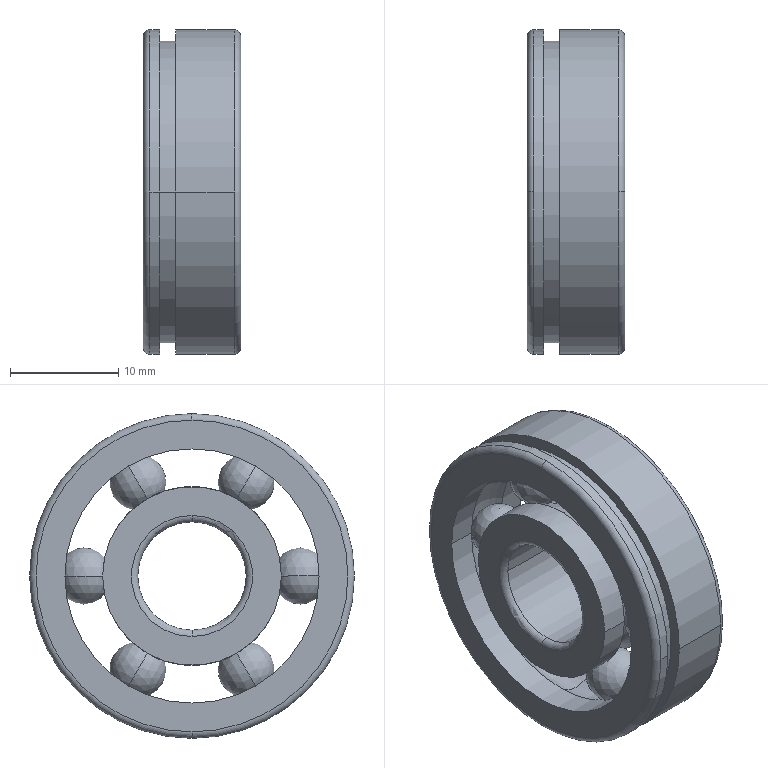Part | SolidWorks | features BaseBody 8 | 8 solids | 48 faces | box 9 x 30 x 30 mm | volume 3673 mm3 | cylinder 16 | torus 14 | sphere 12 | plane 6 | commonest cylinder face diameters 16.52 x4 23.48 x4 30 x4 10 x2 27.84 x2
STEP:
#1=CARTESIAN_POINT('',(4.5,7.4,0.));
#2=VERTEX_POINT('',#1);
#3=CARTESIAN_POINT('',(4.5,12.6,0.));
#4=VERTEX_POINT('',#3);
#5=CARTESIAN_POINT('',(4.5,10.,0.));
#6=DIRECTION('',(0.,0.,1.));
#7=DIRECTION('',(1.,0.,0.));
#8=AXIS2_PLACEMENT_3D('',#5,#6,#7);
#9=CIRCLE('',#8,2.6);
#10=EDGE_CURVE('',#2,#4,#9,.T.);
#11=ORIENTED_EDGE('',*,*,#10,.F.);
#12=CARTESIAN_POINT('',(4.5,10.,0.));
#13=DIRECTION('',(0.,0.,-1.));
#14=DIRECTION('',(-1.,0.,0.));
#15=AXIS2_PLACEMENT_3D('',#12,#13,#14);
#16=CIRCLE('',#15,2.6);
#17=EDGE_CURVE('',#2,#4,#16,.T.);
#18=ORIENTED_EDGE('',*,*,#17,.T.);
#19=EDGE_LOOP('',(#11,#18));
#20=FACE_OUTER_BOUND('',#19,.T.);
#21=CARTESIAN_POINT('',(4.5,10.,0.));
#22=DIRECTION('',(0.,0.,-1.));
#23=DIRECTION('',(1.,0.,0.));
#24=AXIS2_PLACEMENT_3D('',#21,#22,#23);
#25=SPHERICAL_SURFACE('',#24,2.6);
#26=ADVANCED_FACE('',(#20),#25,.T.);
#27=ORIENTED_EDGE('',*,*,#17,.F.);
#28=ORIENTED_EDGE('',*,*,#10,.T.);
#29=EDGE_LOOP('',(#27,#28));
#30=FACE_OUTER_BOUND('',#29,.T.);
#31=CARTESIAN_POINT('',(4.5,10.,0.));
#32=DIRECTION('',(0.,0.,-1.));
#33=DIRECTION('',(1.,0.,0.));
#34=AXIS2_PLACEMENT_3D('',#31,#32,#33);
#35=SPHERICAL_SURFACE('',#34,2.6);
#36=ADVANCED_FACE('',(#30),#35,.T.);
#37=CLOSED_SHELL('',(#26,#36));
#38=MANIFOLD_SOLID_BREP('',#37);
#39=CARTESIAN_POINT('',(3.,-13.92,0.));
#40=VERTEX_POINT('',#39);
#41=CARTESIAN_POINT('',(3.,13.92,0.));
#42=VERTEX_POINT('',#41);
#43=CARTESIAN_POINT('',(3.,0.,0.));
#44=DIRECTION('',(1.,0.,0.));
#45=DIRECTION('',(0.,1.,0.));
#46=AXIS2_PLACEMENT_3D('',#43,#44,#45);
#47=CIRCLE('',#46,13.92);
#48=EDGE_CURVE('',#40,#42,#47,.T.);
#49=ORIENTED_EDGE('',*,*,#48,.F.);
#50=CARTESIAN_POINT('',(1.5,-13.92,0.));
#51=VERTEX_POINT('',#50);
#52=CARTESIAN_POINT('',(2.25,-13.92,0.));
#53=DIRECTION('',(-1.,0.,0.));
#54=VECTOR('',#53,1000.);
#55=LINE('',#52,#54);
#56=EDGE_CURVE('',#40,#51,#55,.T.);
#57=ORIENTED_EDGE('',*,*,#56,.T.);
#58=CARTESIAN_POINT('',(1.5,13.92,0.));
#59=VERTEX_POINT('',#58);
#60=CARTESIAN_POINT('',(1.5,0.,0.));
#61=DIRECTION('',(1.,0.,0.));
#62=DIRECTION('',(0.,1.,0.));
#63=AXIS2_PLACEMENT_3D('',#60,#61,#62);
#64=CIRCLE('',#63,13.92);
#65=EDGE_CURVE('',#51,#59,#64,.T.);
#66=ORIENTED_EDGE('',*,*,#65,.T.);
#67=CARTESIAN_POINT('',(2.25,13.92,0.));
#68=DIRECTION('',(-1.,0.,0.));
#69=VECTOR('',#68,1000.);
#70=LINE('',#67,#69);
#71=EDGE_CURVE('',#42,#59,#70,.T.);
#72=ORIENTED_EDGE('',*,*,#71,.F.);
#73=EDGE_LOOP('',(#49,#57,#66,#72));
#74=FACE_OUTER_BOUND('',#73,.T.);
#75=CARTESIAN_POINT('',(2.25,0.,0.));
#76=DIRECTION('',(-1.,0.,0.));
#77=DIRECTION('',(0.,1.,0.));
#78=AXIS2_PLACEMENT_3D('',#75,#76,#77);
#79=CYLINDRICAL_SURFACE('',#78,13.92);
#80=ADVANCED_FACE('',(#74),#79,.T.);
#81=CARTESIAN_POINT('',(8.4,-15.,0.));
#82=VERTEX_POINT('',#81);
#83=CARTESIAN_POINT('',(8.4,0.,-15.));
#84=VERTEX_POINT('',#83);
#85=CARTESIAN_POINT('',(8.4,0.,0.));
#86=DIRECTION('',(1.,0.,0.));
#87=DIRECTION('',(0.,-1.,0.));
#88=AXIS2_PLACEMENT_3D('',#85,#86,#87);
#89=CIRCLE('',#88,15.);
#90=EDGE_CURVE('',#82,#84,#89,.T.);
#91=ORIENTED_EDGE('',*,*,#90,.F.);
#92=CARTESIAN_POINT('',(3.,-15.,0.));
#93=VERTEX_POINT('',#92);
#94=CARTESIAN_POINT('',(6.,-15.,0.));
#95=DIRECTION('',(-1.,0.,0.));
#96=VECTOR('',#95,1000.);
#97=LINE('',#94,#96);
#98=EDGE_CURVE('',#82,#93,#97,.T.);
#99=ORIENTED_EDGE('',*,*,#98,.T.);
#100=CARTESIAN_POINT('',(3.,15.,0.));
#101=VERTEX_POINT('',#100);
#102=CARTESIAN_POINT('',(3.,0.,0.));
#103=DIRECTION('',(1.,0.,0.));
#104=DIRECTION('',(0.,1.,0.));
#105=AXIS2_PLACEMENT_3D('',#102,#103,#104);
#106=CIRCLE('',#105,15.);
#107=EDGE_CURVE('',#93,#101,#106,.T.);
#108=ORIENTED_EDGE('',*,*,#107,.T.);
#109=CARTESIAN_POINT('',(8.4,15.,0.));
#110=VERTEX_POINT('',#109);
#111=CARTESIAN_POINT('',(6.,15.,0.));
#112=DIRECTION('',(-1.,0.,0.));
#113=VECTOR('',#112,1000.);
#114=LINE('',#111,#113);
#115=EDGE_CURVE('',#110,#101,#114,.T.);
#116=ORIENTED_EDGE('',*,*,#115,.F.);
#117=CARTESIAN_POINT('',(8.4,0.,0.));
#118=DIRECTION('',(1.,0.,0.));
#119=DIRECTION('',(0.,-1.,0.));
#120=AXIS2_PLACEMENT_3D('',#117,#118,#119);
#121=CIRCLE('',#120,15.);
#122=EDGE_CURVE('',#84,#110,#121,.T.);
#123=ORIENTED_EDGE('',*,*,#122,.F.);
#124=EDGE_LOOP('',(#91,#99,#108,#116,#123));
#125=FACE_OUTER_BOUND('',#124,.T.);
#126=CARTESIAN_POINT('',(6.,0.,0.));
#127=DIRECTION('',(-1.,0.,0.));
#128=DIRECTION('',(0.,1.,0.));
#129=AXIS2_PLACEMENT_3D('',#126,#127,#128);
#130=CYLINDRICAL_SURFACE('',#129,15.);
#131=ADVANCED_FACE('',(#125),#130,.T.);
#132=CARTESIAN_POINT('',(1.5,-15.,0.));
#133=VERTEX_POINT('',#132);
#134=CARTESIAN_POINT('',(1.5,15.,0.));
#135=VERTEX_POINT('',#134);
#136=CARTESIAN_POINT('',(1.5,0.,0.));
#137=DIRECTION('',(1.,0.,0.));
#138=DIRECTION('',(0.,1.,0.));
#139=AXIS2_PLACEMENT_3D('',#136,#137,#138);
#140=CIRCLE('',#139,15.);
#141=EDGE_CURVE('',#133,#135,#140,.T.);
#142=ORIENTED_EDGE('',*,*,#141,.F.);
#143=CARTESIAN_POINT('',(0.6,-15.,0.));
#144=VERTEX_POINT('',#143);
#145=CARTESIAN_POINT('',(0.75,-15.,0.));
#146=DIRECTION('',(-1.,0.,0.));
#147=VECTOR('',#146,1000.);
#148=LINE('',#145,#147);
#149=EDGE_CURVE('',#133,#144,#148,.T.);
#150=ORIENTED_EDGE('',*,*,#149,.T.);
#151=CARTESIAN_POINT('',(0.6,0.,-15.));
#152=VERTEX_POINT('',#151);
#153=CARTESIAN_POINT('',(0.6,0.,0.));
#154=DIRECTION('',(-1.,0.,0.));
#155=DIRECTION('',(0.,-1.,0.));
#156=AXIS2_PLACEMENT_3D('',#153,#154,#155);
#157=CIRCLE('',#156,15.);
#158=EDGE_CURVE('',#152,#144,#157,.T.);
#159=ORIENTED_EDGE('',*,*,#158,.F.);
#160=CARTESIAN_POINT('',(0.6,15.,0.));
#161=VERTEX_POINT('',#160);
#162=CARTESIAN_POINT('',(0.6,0.,0.));
#163=DIRECTION('',(-1.,0.,0.));
#164=DIRECTION('',(0.,-1.,0.));
#165=AXIS2_PLACEMENT_3D('',#162,#163,#164);
#166=CIRCLE('',#165,15.);
#167=EDGE_CURVE('',#161,#152,#166,.T.);
#168=ORIENTED_EDGE('',*,*,#167,.F.);
#169=CARTESIAN_POINT('',(0.75,15.,0.));
#170=DIRECTION('',(-1.,0.,0.));
#171=VECTOR('',#170,1000.);
#172=LINE('',#169,#171);
#173=EDGE_CURVE('',#135,#161,#172,.T.);
#174=ORIENTED_EDGE('',*,*,#173,.F.);
#175=EDGE_LOOP('',(#142,#150,#159,#168,#174));
#176=FACE_OUTER_BOUND('',#175,.T.);
#177=CARTESIAN_POINT('',(0.75,0.,0.));
#178=DIRECTION('',(-1.,0.,0.));
#179=DIRECTION('',(0.,1.,0.));
#180=AXIS2_PLACEMENT_3D('',#177,#178,#179);
#181=CYLINDRICAL_SURFACE('',#180,15.);
#182=ADVANCED_FACE('',(#176),#181,.T.);
#183=ORIENTED_EDGE('',*,*,#122,.T.);
#184=CARTESIAN_POINT('',(8.4,0.,15.));
#185=VERTEX_POINT('',#184);
#186=CARTESIAN_POINT('',(8.4,0.,0.));
#187=DIRECTION('',(1.,0.,0.));
#188=DIRECTION('',(0.,-1.,0.));
#189=AXIS2_PLACEMENT_3D('',#186,#187,#188);
#190=CIRCLE('',#189,15.);
#191=EDGE_CURVE('',#110,#185,#190,.T.);
#192=ORIENTED_EDGE('',*,*,#191,.T.);
#193=CARTESIAN_POINT('',(9.,0.,14.4));
#194=VERTEX_POINT('',#193);
#195=CARTESIAN_POINT('',(8.4,0.,14.4));
#196=DIRECTION('',(0.,1.,0.));
#197=DIRECTION('',(0.,0.,1.));
#198=AXIS2_PLACEMENT_3D('',#195,#196,#197);
#199=CIRCLE('',#198,0.6);
#200=EDGE_CURVE('',#185,#194,#199,.T.);
#201=ORIENTED_EDGE('',*,*,#200,.T.);
#202=CARTESIAN_POINT('',(9.,0.,-14.4));
#203=VERTEX_POINT('',#202);
#204=CARTESIAN_POINT('',(9.,0.,0.));
#205=DIRECTION('',(-1.,0.,0.));
#206=DIRECTION('',(0.,-1.,0.));
#207=AXIS2_PLACEMENT_3D('',#204,#205,#206);
#208=CIRCLE('',#207,14.4);
#209=EDGE_CURVE('',#194,#203,#208,.T.);
#210=ORIENTED_EDGE('',*,*,#209,.T.);
#211=CARTESIAN_POINT('',(8.4,0.,-14.4));
#212=DIRECTION('',(0.,-1.,0.));
#213=DIRECTION('',(0.,0.,-1.));
#214=AXIS2_PLACEMENT_3D('',#211,#212,#213);
#215=CIRCLE('',#214,0.6);
#216=EDGE_CURVE('',#84,#203,#215,.T.);
#217=ORIENTED_EDGE('',*,*,#216,.F.);
#218=EDGE_LOOP('',(#183,#192,#201,#210,#217));
#219=FACE_OUTER_BOUND('',#218,.T.);
#220=CARTESIAN_POINT('',(8.4,0.,0.));
#221=DIRECTION('',(1.,0.,0.));
#222=DIRECTION('',(0.,0.,-1.));
#223=AXIS2_PLACEMENT_3D('',#220,#221,#222);
#224=TOROIDAL_SURFACE('',#223,14.4,0.6);
#225=ADVANCED_FACE('',(#219),#224,.T.);
#226=CARTESIAN_POINT('',(0.,0.,-14.4));
#227=VERTEX_POINT('',#226);
#228=CARTESIAN_POINT('',(0.,0.,14.4));
#229=VERTEX_POINT('',#228);
#230=CARTESIAN_POINT('',(0.,0.,0.));
#231=DIRECTION('',(1.,0.,0.));
#232=DIRECTION('',(0.,-1.,0.));
#233=AXIS2_PLACEMENT_3D('',#230,#231,#232);
#234=CIRCLE('',#233,14.4);
#235=EDGE_CURVE('',#227,#229,#234,.T.);
#236=ORIENTED_EDGE('',*,*,#235,.T.);
#237=CARTESIAN_POINT('',(0.6,0.,15.));
#238=VERTEX_POINT('',#237);
#239=CARTESIAN_POINT('',(0.6,0.,14.4));
#240=DIRECTION('',(0.,1.,0.));
#241=DIRECTION('',(0.,0.,1.));
#242=AXIS2_PLACEMENT_3D('',#239,#240,#241);
#243=CIRCLE('',#242,0.6);
#244=EDGE_CURVE('',#229,#238,#243,.T.);
#245=ORIENTED_EDGE('',*,*,#244,.T.);
#246=CARTESIAN_POINT('',(0.6,0.,0.));
#247=DIRECTION('',(-1.,0.,0.));
#248=DIRECTION('',(0.,-1.,0.));
#249=AXIS2_PLACEMENT_3D('',#246,#247,#248);
#250=CIRCLE('',#249,15.);
#251=EDGE_CURVE('',#238,#161,#250,.T.);
#252=ORIENTED_EDGE('',*,*,#251,.T.);
#253=ORIENTED_EDGE('',*,*,#167,.T.);
#254=CARTESIAN_POINT('',(0.6,0.,-14.4));
#255=DIRECTION('',(0.,-1.,0.));
#256=DIRECTION('',(0.,0.,-1.));
#257=AXIS2_PLACEMENT_3D('',#254,#255,#256);
#258=CIRCLE('',#257,0.6);
#259=EDGE_CURVE('',#227,#152,#258,.T.);
#260=ORIENTED_EDGE('',*,*,#259,.F.);
#261=EDGE_LOOP('',(#236,#245,#252,#253,#260));
#262=FACE_OUTER_BOUND('',#261,.T.);
#263=CARTESIAN_POINT('',(0.6,0.,0.));
#264=DIRECTION('',(1.,0.,0.));
#265=DIRECTION('',(0.,0.,-1.));
#266=AXIS2_PLACEMENT_3D('',#263,#264,#265);
#267=TOROIDAL_SURFACE('',#266,14.4,0.6);
#268=ADVANCED_FACE('',(#262),#267,.T.);
#269=CARTESIAN_POINT('',(2.568,0.,11.74));
#270=VERTEX_POINT('',#269);
#271=CARTESIAN_POINT('',(2.568,-11.74,0.));
#272=VERTEX_POINT('',#271);
#273=CARTESIAN_POINT('',(2.568,0.,0.));
#274=DIRECTION('',(1.,0.,0.));
#275=DIRECTION('',(0.,1.,0.));
#276=AXIS2_PLACEMENT_3D('',#273,#274,#275);
#277=CIRCLE('',#276,11.74);
#278=EDGE_CURVE('',#270,#272,#277,.T.);
#279=ORIENTED_EDGE('',*,*,#278,.F.);
#280=CARTESIAN_POINT('',(6.432,0.,11.74));
#281=VERTEX_POINT('',#280);
#282=CARTESIAN_POINT('',(4.5,0.,10.));
#283=DIRECTION('',(0.,1.,0.));
#284=DIRECTION('',(0.,0.,1.));
#285=AXIS2_PLACEMENT_3D('',#282,#283,#284);
#286=CIRCLE('',#285,2.6);
#287=EDGE_CURVE('',#270,#281,#286,.T.);
#288=ORIENTED_EDGE('',*,*,#287,.T.);
#289=CARTESIAN_POINT('',(6.432,-11.74,0.));
#290=VERTEX_POINT('',#289);
#291=CARTESIAN_POINT('',(6.432,0.,0.));
#292=DIRECTION('',(1.,0.,0.));
#293=DIRECTION('',(0.,1.,0.));
#294=AXIS2_PLACEMENT_3D('',#291,#292,#293);
#295=CIRCLE('',#294,11.74);
#296=EDGE_CURVE('',#281,#290,#295,.T.);
#297=ORIENTED_EDGE('',*,*,#296,.T.);
#298=CARTESIAN_POINT('',(6.432,0.,-11.74));
#299=VERTEX_POINT('',#298);
#300=CARTESIAN_POINT('',(6.432,0.,0.));
#301=DIRECTION('',(1.,0.,0.));
#302=DIRECTION('',(0.,1.,0.));
#303=AXIS2_PLACEMENT_3D('',#300,#301,#302);
#304=CIRCLE('',#303,11.74);
#305=EDGE_CURVE('',#290,#299,#304,.T.);
#306=ORIENTED_EDGE('',*,*,#305,.T.);
#307=CARTESIAN_POINT('',(2.568,0.,-11.74));
#308=VERTEX_POINT('',#307);
#309=CARTESIAN_POINT('',(4.5,0.,-10.));
#310=DIRECTION('',(0.,-1.,0.));
#311=DIRECTION('',(0.,0.,-1.));
#312=AXIS2_PLACEMENT_3D('',#309,#310,#311);
#313=CIRCLE('',#312,2.6);
#314=EDGE_CURVE('',#308,#299,#313,.T.);
#315=ORIENTED_EDGE('',*,*,#314,.F.);
#316=CARTESIAN_POINT('',(2.568,0.,0.));
#317=DIRECTION('',(1.,0.,0.));
#318=DIRECTION('',(0.,1.,0.));
#319=AXIS2_PLACEMENT_3D('',#316,#317,#318);
#320=CIRCLE('',#319,11.74);
#321=EDGE_CURVE('',#272,#308,#320,.T.);
#322=ORIENTED_EDGE('',*,*,#321,.F.);
#323=EDGE_LOOP('',(#279,#288,#297,#306,#315,#322));
#324=FACE_OUTER_BOUND('',#323,.T.);
#325=CARTESIAN_POINT('',(4.5,0.,0.));
#326=DIRECTION('',(1.,0.,0.));
#327=DIRECTION('',(0.,0.,-1.));
#328=AXIS2_PLACEMENT_3D('',#325,#326,#327);
#329=TOROIDAL_SURFACE('',#328,10.,2.6);
#330=ADVANCED_FACE('',(#324),#329,.F.);
#331=CARTESIAN_POINT('',(9.,11.74,0.));
#332=VERTEX_POINT('',#331);
#333=CARTESIAN_POINT('',(9.,-11.74,0.));
#334=VERTEX_POINT('',#333);
#335=CARTESIAN_POINT('',(9.,0.,0.));
#336=DIRECTION('',(1.,0.,0.));
#337=DIRECTION('',(0.,1.,0.));
#338=AXIS2_PLACEMENT_3D('',#335,#336,#337);
#339=CIRCLE('',#338,11.74);
#340=EDGE_CURVE('',#332,#334,#339,.T.);
#341=ORIENTED_EDGE('',*,*,#340,.T.);
#342=CARTESIAN_POINT('',(7.716,-11.74,0.));
#343=DIRECTION('',(-1.,0.,0.));
#344=VECTOR('',#343,1000.);
#345=LINE('',#342,#344);
#346=EDGE_CURVE('',#334,#290,#345,.T.);
#347=ORIENTED_EDGE('',*,*,#346,.T.);
#348=ORIENTED_EDGE('',*,*,#296,.F.);
#349=CARTESIAN_POINT('',(6.432,11.74,0.));
#350=VERTEX_POINT('',#349);
#351=CARTESIAN_POINT('',(6.432,0.,0.));
#352=DIRECTION('',(1.,0.,0.));
#353=DIRECTION('',(0.,1.,0.));
#354=AXIS2_PLACEMENT_3D('',#351,#352,#353);
#355=CIRCLE('',#354,11.74);
#356=EDGE_CURVE('',#350,#281,#355,.T.);
#357=ORIENTED_EDGE('',*,*,#356,.F.);
#358=CARTESIAN_POINT('',(7.716,11.74,0.));
#359=DIRECTION('',(-1.,0.,0.));
#360=VECTOR('',#359,1000.);
#361=LINE('',#358,#360);
#362=EDGE_CURVE('',#332,#350,#361,.T.);
#363=ORIENTED_EDGE('',*,*,#362,.F.);
#364=EDGE_LOOP('',(#341,#347,#348,#357,#363));
#365=FACE_OUTER_BOUND('',#364,.T.);
#366=CARTESIAN_POINT('',(7.716,0.,0.));
#367=DIRECTION('',(-1.,0.,0.));
#368=DIRECTION('',(0.,1.,0.));
#369=AXIS2_PLACEMENT_3D('',#366,#367,#368);
#370=CYLINDRICAL_SURFACE('',#369,11.74);
#371=ADVANCED_FACE('',(#365),#370,.F.);
#372=CARTESIAN_POINT('',(2.568,11.74,0.));
#373=VERTEX_POINT('',#372);
#374=CARTESIAN_POINT('',(2.568,0.,0.));
#375=DIRECTION('',(1.,0.,0.));
#376=DIRECTION('',(0.,1.,0.));
#377=AXIS2_PLACEMENT_3D('',#374,#375,#376);
#378=CIRCLE('',#377,11.74);
#379=EDGE_CURVE('',#373,#270,#378,.T.);
#380=ORIENTED_EDGE('',*,*,#379,.T.);
#381=ORIENTED_EDGE('',*,*,#278,.T.);
#382=CARTESIAN_POINT('',(0.,-11.74,0.));
#383=VERTEX_POINT('',#382);
#384=CARTESIAN_POINT('',(1.284,-11.74,0.));
#385=DIRECTION('',(-1.,0.,0.));
#386=VECTOR('',#385,1000.);
#387=LINE('',#384,#386);
#388=EDGE_CURVE('',#272,#383,#387,.T.);
#389=ORIENTED_EDGE('',*,*,#388,.T.);
#390=CARTESIAN_POINT('',(0.,11.74,0.));
#391=VERTEX_POINT('',#390);
#392=CARTESIAN_POINT('',(0.,0.,0.));
#393=DIRECTION('',(1.,0.,0.));
#394=DIRECTION('',(0.,1.,0.));
#395=AXIS2_PLACEMENT_3D('',#392,#393,#394);
#396=CIRCLE('',#395,11.74);
#397=EDGE_CURVE('',#391,#383,#396,.T.);
#398=ORIENTED_EDGE('',*,*,#397,.F.);
#399=CARTESIAN_POINT('',(1.284,11.74,0.));
#400=DIRECTION('',(-1.,0.,0.));
#401=VECTOR('',#400,1000.);
#402=LINE('',#399,#401);
#403=EDGE_CURVE('',#373,#391,#402,.T.);
#404=ORIENTED_EDGE('',*,*,#403,.F.);
#405=EDGE_LOOP('',(#380,#381,#389,#398,#404));
#406=FACE_OUTER_BOUND('',#405,.T.);
#407=CARTESIAN_POINT('',(1.284,0.,0.));
#408=DIRECTION('',(-1.,0.,0.));
#409=DIRECTION('',(0.,1.,0.));
#410=AXIS2_PLACEMENT_3D('',#407,#408,#409);
#411=CYLINDRICAL_SURFACE('',#410,11.74);
#412=ADVANCED_FACE('',(#406),#411,.F.);
#413=CARTESIAN_POINT('',(3.,0.,0.));
#414=DIRECTION('',(1.,0.,0.));
#415=DIRECTION('',(0.,1.,0.));
#416=AXIS2_PLACEMENT_3D('',#413,#414,#415);
#417=CIRCLE('',#416,13.92);
#418=EDGE_CURVE('',#42,#40,#417,.T.);
#419=ORIENTED_EDGE('',*,*,#418,.T.);
#420=ORIENTED_EDGE('',*,*,#48,.T.);
#421=EDGE_LOOP('',(#419,#420));
#422=FACE_BOUND('',#421,.T.);
#423=CARTESIAN_POINT('',(3.,0.,0.));
#424=DIRECTION('',(1.,0.,0.));
#425=DIRECTION('',(0.,1.,0.));
#426=AXIS2_PLACEMENT_3D('',#423,#424,#425);
#427=CIRCLE('',#426,15.);
#428=EDGE_CURVE('',#101,#93,#427,.T.);
#429=ORIENTED_EDGE('',*,*,#428,.F.);
#430=ORIENTED_EDGE('',*,*,#107,.F.);
#431=EDGE_LOOP('',(#429,#430));
#432=FACE_OUTER_BOUND('',#431,.T.);
#433=CARTESIAN_POINT('',(3.,14.46,0.));
#434=DIRECTION('',(-1.,0.,0.));
#435=DIRECTION('',(0.,0.,1.));
#436=AXIS2_PLACEMENT_3D('',#433,#434,#435);
#437=PLANE('',#436);
#438=ADVANCED_FACE('',(#422,#432),#437,.T.);
#439=CARTESIAN_POINT('',(1.5,0.,0.));
#440=DIRECTION('',(1.,0.,0.));
#441=DIRECTION('',(0.,1.,0.));
#442=AXIS2_PLACEMENT_3D('',#439,#440,#441);
#443=CIRCLE('',#442,13.92);
#444=EDGE_CURVE('',#59,#51,#443,.T.);
#445=ORIENTED_EDGE('',*,*,#444,.F.);
#446=ORIENTED_EDGE('',*,*,#65,.F.);
#447=EDGE_LOOP('',(#445,#446));
#448=FACE_BOUND('',#447,.T.);
#449=CARTESIAN_POINT('',(1.5,0.,0.));
#450=DIRECTION('',(1.,0.,0.));
#451=DIRECTION('',(0.,1.,0.));
#452=AXIS2_PLACEMENT_3D('',#449,#450,#451);
#453=CIRCLE('',#452,15.);
#454=EDGE_CURVE('',#135,#133,#453,.T.);
#455=ORIENTED_EDGE('',*,*,#454,.T.);
#456=ORIENTED_EDGE('',*,*,#141,.T.);
#457=EDGE_LOOP('',(#455,#456));
#458=FACE_OUTER_BOUND('',#457,.T.);
#459=CARTESIAN_POINT('',(1.5,14.46,0.));
#460=DIRECTION('',(1.,0.,0.));
#461=DIRECTION('',(0.,1.,0.));
#462=AXIS2_PLACEMENT_3D('',#459,#460,#461);
#463=PLANE('',#462);
#464=ADVANCED_FACE('',(#448,#458),#463,.T.);
#465=ORIENTED_EDGE('',*,*,#340,.F.);
#466=CARTESIAN_POINT('',(9.,0.,0.));
#467=DIRECTION('',(1.,0.,0.));
#468=DIRECTION('',(0.,1.,0.));
#469=AXIS2_PLACEMENT_3D('',#466,#467,#468);
#470=CIRCLE('',#469,11.74);
#471=EDGE_CURVE('',#334,#332,#470,.T.);
#472=ORIENTED_EDGE('',*,*,#471,.F.);
#473=EDGE_LOOP('',(#465,#472));
#474=FACE_BOUND('',#473,.T.);
#475=CARTESIAN_POINT('',(9.,0.,0.));
#476=DIRECTION('',(-1.,0.,0.));
#477=DIRECTION('',(0.,-1.,0.));
#478=AXIS2_PLACEMENT_3D('',#475,#476,#477);
#479=CIRCLE('',#478,14.4);
#480=EDGE_CURVE('',#203,#194,#479,.T.);
#481=ORIENTED_EDGE('',*,*,#480,.F.);
#482=ORIENTED_EDGE('',*,*,#209,.F.);
#483=EDGE_LOOP('',(#481,#482));
#484=FACE_OUTER_BOUND('',#483,.T.);
#485=CARTESIAN_POINT('',(9.,13.37,0.));
#486=DIRECTION('',(1.,0.,0.));
#487=DIRECTION('',(0.,1.,0.));
#488=AXIS2_PLACEMENT_3D('',#485,#486,#487);
#489=PLANE('',#488);
#490=ADVANCED_FACE('',(#474,#484),#489,.T.);
#491=ORIENTED_EDGE('',*,*,#397,.T.);
#492=CARTESIAN_POINT('',(0.,0.,0.));
#493=DIRECTION('',(1.,0.,0.));
#494=DIRECTION('',(0.,1.,0.));
#495=AXIS2_PLACEMENT_3D('',#492,#493,#494);
#496=CIRCLE('',#495,11.74);
#497=EDGE_CURVE('',#383,#391,#496,.T.);
#498=ORIENTED_EDGE('',*,*,#497,.T.);
#499=EDGE_LOOP('',(#491,#498));
#500=FACE_BOUND('',#499,.T.);
#501=ORIENTED_EDGE('',*,*,#235,.F.);
#502=CARTESIAN_POINT('',(0.,0.,0.));
#503=DIRECTION('',(1.,0.,0.));
#504=DIRECTION('',(0.,-1.,0.));
#505=AXIS2_PLACEMENT_3D('',#502,#503,#504);
#506=CIRCLE('',#505,14.4);
#507=EDGE_CURVE('',#229,#227,#506,.T.);
#508=ORIENTED_EDGE('',*,*,#507,.F.);
#509=EDGE_LOOP('',(#501,#508));
#510=FACE_OUTER_BOUND('',#509,.T.);
#511=CARTESIAN_POINT('',(0.,13.37,0.));
#512=DIRECTION('',(-1.,0.,0.));
#513=DIRECTION('',(0.,0.,1.));
#514=AXIS2_PLACEMENT_3D('',#511,#512,#513);
#515=PLANE('',#514);
#516=ADVANCED_FACE('',(#500,#510),#515,.T.);
#517=ORIENTED_EDGE('',*,*,#388,.F.);
#518=ORIENTED_EDGE('',*,*,#321,.T.);
#519=CARTESIAN_POINT('',(2.568,0.,0.));
#520=DIRECTION('',(1.,0.,0.));
#521=DIRECTION('',(0.,1.,0.));
#522=AXIS2_PLACEMENT_3D('',#519,#520,#521);
#523=CIRCLE('',#522,11.74);
#524=EDGE_CURVE('',#308,#373,#523,.T.);
#525=ORIENTED_EDGE('',*,*,#524,.T.);
#526=ORIENTED_EDGE('',*,*,#403,.T.);
#527=ORIENTED_EDGE('',*,*,#497,.F.);
#528=EDGE_LOOP('',(#517,#518,#525,#526,#527));
#529=FACE_OUTER_BOUND('',#528,.T.);
#530=CARTESIAN_POINT('',(1.284,0.,0.));
#531=DIRECTION('',(-1.,0.,0.));
#532=DIRECTION('',(0.,1.,0.));
#533=AXIS2_PLACEMENT_3D('',#530,#531,#532);
#534=CYLINDRICAL_SURFACE('',#533,11.74);
#535=ADVANCED_FACE('',(#529),#534,.F.);
#536=ORIENTED_EDGE('',*,*,#346,.F.);
#537=ORIENTED_EDGE('',*,*,#471,.T.);
#538=ORIENTED_EDGE('',*,*,#362,.T.);
#539=CARTESIAN_POINT('',(6.432,0.,0.));
#540=DIRECTION('',(1.,0.,0.));
#541=DIRECTION('',(0.,1.,0.));
#542=AXIS2_PLACEMENT_3D('',#539,#540,#541);
#543=CIRCLE('',#542,11.74);
#544=EDGE_CURVE('',#299,#350,#543,.T.);
#545=ORIENTED_EDGE('',*,*,#544,.F.);
#546=ORIENTED_EDGE('',*,*,#305,.F.);
#547=EDGE_LOOP('',(#536,#537,#538,#545,#546));
#548=FACE_OUTER_BOUND('',#547,.T.);
#549=CARTESIAN_POINT('',(7.716,0.,0.));
#550=DIRECTION('',(-1.,0.,0.));
#551=DIRECTION('',(0.,1.,0.));
#552=AXIS2_PLACEMENT_3D('',#549,#550,#551);
#553=CYLINDRICAL_SURFACE('',#552,11.74);
#554=ADVANCED_FACE('',(#548),#553,.F.);
#555=ORIENTED_EDGE('',*,*,#287,.F.);
#556=ORIENTED_EDGE('',*,*,#379,.F.);
#557=ORIENTED_EDGE('',*,*,#524,.F.);
#558=ORIENTED_EDGE('',*,*,#314,.T.);
#559=ORIENTED_EDGE('',*,*,#544,.T.);
#560=ORIENTED_EDGE('',*,*,#356,.T.);
#561=EDGE_LOOP('',(#555,#556,#557,#558,#559,#560));
#562=FACE_OUTER_BOUND('',#561,.T.);
#563=CARTESIAN_POINT('',(4.5,0.,0.));
#564=DIRECTION('',(1.,0.,0.));
#565=DIRECTION('',(0.,0.,-1.));
#566=AXIS2_PLACEMENT_3D('',#563,#564,#565);
#567=TOROIDAL_SURFACE('',#566,10.,2.6);
#568=ADVANCED_FACE('',(#562),#567,.F.);
#569=ORIENTED_EDGE('',*,*,#244,.F.);
#570=ORIENTED_EDGE('',*,*,#507,.T.);
#571=ORIENTED_EDGE('',*,*,#259,.T.);
#572=ORIENTED_EDGE('',*,*,#158,.T.);
#573=CARTESIAN_POINT('',(0.6,0.,0.));
#574=DIRECTION('',(-1.,0.,0.));
#575=DIRECTION('',(0.,-1.,0.));
#576=AXIS2_PLACEMENT_3D('',#573,#574,#575);
#577=CIRCLE('',#576,15.);
#578=EDGE_CURVE('',#144,#238,#577,.T.);
#579=ORIENTED_EDGE('',*,*,#578,.T.);
#580=EDGE_LOOP('',(#569,#570,#571,#572,#579));
#581=FACE_OUTER_BOUND('',#580,.T.);
#582=CARTESIAN_POINT('',(0.6,0.,0.));
#583=DIRECTION('',(1.,0.,0.));
#584=DIRECTION('',(0.,0.,-1.));
#585=AXIS2_PLACEMENT_3D('',#582,#583,#584);
#586=TOROIDAL_SURFACE('',#585,14.4,0.6);
#587=ADVANCED_FACE('',(#581),#586,.T.);
#588=ORIENTED_EDGE('',*,*,#200,.F.);
#589=CARTESIAN_POINT('',(8.4,0.,0.));
#590=DIRECTION('',(1.,0.,0.));
#591=DIRECTION('',(0.,-1.,0.));
#592=AXIS2_PLACEMENT_3D('',#589,#590,#591);
#593=CIRCLE('',#592,15.);
#594=EDGE_CURVE('',#185,#82,#593,.T.);
#595=ORIENTED_EDGE('',*,*,#594,.T.);
#596=ORIENTED_EDGE('',*,*,#90,.T.);
#597=ORIENTED_EDGE('',*,*,#216,.T.);
#598=ORIENTED_EDGE('',*,*,#480,.T.);
#599=EDGE_LOOP('',(#588,#595,#596,#597,#598));
#600=FACE_OUTER_BOUND('',#599,.T.);
#601=CARTESIAN_POINT('',(8.4,0.,0.));
#602=DIRECTION('',(1.,0.,0.));
#603=DIRECTION('',(0.,0.,-1.));
#604=AXIS2_PLACEMENT_3D('',#601,#602,#603);
#605=TOROIDAL_SURFACE('',#604,14.4,0.6);
#606=ADVANCED_FACE('',(#600),#605,.T.);
#607=ORIENTED_EDGE('',*,*,#149,.F.);
#608=ORIENTED_EDGE('',*,*,#454,.F.);
#609=ORIENTED_EDGE('',*,*,#173,.T.);
#610=ORIENTED_EDGE('',*,*,#251,.F.);
#611=ORIENTED_EDGE('',*,*,#578,.F.);
#612=EDGE_LOOP('',(#607,#608,#609,#610,#611));
#613=FACE_OUTER_BOUND('',#612,.T.);
#614=CARTESIAN_POINT('',(0.75,0.,0.));
#615=DIRECTION('',(-1.,0.,0.));
#616=DIRECTION('',(0.,1.,0.));
#617=AXIS2_PLACEMENT_3D('',#614,#615,#616);
#618=CYLINDRICAL_SURFACE('',#617,15.);
#619=ADVANCED_FACE('',(#613),#618,.T.);
#620=ORIENTED_EDGE('',*,*,#98,.F.);
#621=ORIENTED_EDGE('',*,*,#594,.F.);
#622=ORIENTED_EDGE('',*,*,#191,.F.);
#623=ORIENTED_EDGE('',*,*,#115,.T.);
#624=ORIENTED_EDGE('',*,*,#428,.T.);
#625=EDGE_LOOP('',(#620,#621,#622,#623,#624));
#626=FACE_OUTER_BOUND('',#625,.T.);
#627=CARTESIAN_POINT('',(6.,0.,0.));
#628=DIRECTION('',(-1.,0.,0.));
#629=DIRECTION('',(0.,1.,0.));
#630=AXIS2_PLACEMENT_3D('',#627,#628,#629);
#631=CYLINDRICAL_SURFACE('',#630,15.);
#632=ADVANCED_FACE('',(#626),#631,.T.);
#633=ORIENTED_EDGE('',*,*,#56,.F.);
#634=ORIENTED_EDGE('',*,*,#418,.F.);
#635=ORIENTED_EDGE('',*,*,#71,.T.);
#636=ORIENTED_EDGE('',*,*,#444,.T.);
#637=EDGE_LOOP('',(#633,#634,#635,#636));
#638=FACE_OUTER_BOUND('',#637,.T.);
#639=CARTESIAN_POINT('',(2.25,0.,0.));
#640=DIRECTION('',(-1.,0.,0.));
#641=DIRECTION('',(0.,1.,0.));
#642=AXIS2_PLACEMENT_3D('',#639,#640,#641);
#643=CYLINDRICAL_SURFACE('',#642,13.92);
#644=ADVANCED_FACE('',(#638),#643,.T.);
#645=CLOSED_SHELL('',(#80,#131,#182,#225,#268,#330,#371,#412,#438,#464,#490,#516,#535,#554,#568,#587,#606,#619,#632,#644));
#646=MANIFOLD_SOLID_BREP('',#645);
#647=CARTESIAN_POINT('',(6.432,0.,-8.26));
#648=VERTEX_POINT('',#647);
#649=CARTESIAN_POINT('',(4.5,0.,-7.4));
#650=VERTEX_POINT('',#649);
#651=CARTESIAN_POINT('',(4.5,0.,-10.));
#652=DIRECTION('',(0.,-1.,0.));
#653=DIRECTION('',(0.,0.,-1.));
#654=AXIS2_PLACEMENT_3D('',#651,#652,#653);
#655=CIRCLE('',#654,2.6);
#656=EDGE_CURVE('',#648,#650,#655,.T.);
#657=ORIENTED_EDGE('',*,*,#656,.T.);
#658=CARTESIAN_POINT('',(4.5,0.,7.4));
#659=VERTEX_POINT('',#658);
#660=CARTESIAN_POINT('',(4.5,0.,0.));
#661=DIRECTION('',(1.,0.,0.));
#662=DIRECTION('',(0.,0.,-1.));
#663=AXIS2_PLACEMENT_3D('',#660,#661,#662);
#664=CIRCLE('',#663,7.4);
#665=EDGE_CURVE('',#650,#659,#664,.T.);
#666=ORIENTED_EDGE('',*,*,#665,.T.);
#667=CARTESIAN_POINT('',(6.432,0.,8.26));
#668=VERTEX_POINT('',#667);
#669=CARTESIAN_POINT('',(4.5,0.,10.));
#670=DIRECTION('',(0.,1.,0.));
#671=DIRECTION('',(0.,0.,1.));
#672=AXIS2_PLACEMENT_3D('',#669,#670,#671);
#673=CIRCLE('',#672,2.6);
#674=EDGE_CURVE('',#668,#659,#673,.T.);
#675=ORIENTED_EDGE('',*,*,#674,.F.);
#676=CARTESIAN_POINT('',(6.432,8.26,0.));
#677=VERTEX_POINT('',#676);
#678=CARTESIAN_POINT('',(6.432,0.,0.));
#679=DIRECTION('',(1.,0.,0.));
#680=DIRECTION('',(0.,1.,0.));
#681=AXIS2_PLACEMENT_3D('',#678,#679,#680);
#682=CIRCLE('',#681,8.26);
#683=EDGE_CURVE('',#677,#668,#682,.T.);
#684=ORIENTED_EDGE('',*,*,#683,.F.);
#685=CARTESIAN_POINT('',(6.432,0.,0.));
#686=DIRECTION('',(1.,0.,0.));
#687=DIRECTION('',(0.,1.,0.));
#688=AXIS2_PLACEMENT_3D('',#685,#686,#687);
#689=CIRCLE('',#688,8.26);
#690=EDGE_CURVE('',#648,#677,#689,.T.);
#691=ORIENTED_EDGE('',*,*,#690,.F.);
#692=EDGE_LOOP('',(#657,#666,#675,#684,#691));
#693=FACE_OUTER_BOUND('',#692,.T.);
#694=CARTESIAN_POINT('',(4.5,0.,0.));
#695=DIRECTION('',(1.,0.,0.));
#696=DIRECTION('',(0.,0.,-1.));
#697=AXIS2_PLACEMENT_3D('',#694,#695,#696);
#698=TOROIDAL_SURFACE('',#697,10.,2.6);
#699=ADVANCED_FACE('',(#693),#698,.F.);
#700=ORIENTED_EDGE('',*,*,#674,.T.);
#701=CARTESIAN_POINT('',(4.5,0.,0.));
#702=DIRECTION('',(1.,0.,0.));
#703=DIRECTION('',(0.,0.,-1.));
#704=AXIS2_PLACEMENT_3D('',#701,#702,#703);
#705=CIRCLE('',#704,7.4);
#706=EDGE_CURVE('',#659,#650,#705,.T.);
#707=ORIENTED_EDGE('',*,*,#706,.T.);
#708=ORIENTED_EDGE('',*,*,#656,.F.);
#709=CARTESIAN_POINT('',(6.432,-8.26,0.));
#710=VERTEX_POINT('',#709);
#711=CARTESIAN_POINT('',(6.432,0.,0.));
#712=DIRECTION('',(1.,0.,0.));
#713=DIRECTION('',(0.,1.,0.));
#714=AXIS2_PLACEMENT_3D('',#711,#712,#713);
#715=CIRCLE('',#714,8.26);
#716=EDGE_CURVE('',#710,#648,#715,.T.);
#717=ORIENTED_EDGE('',*,*,#716,.F.);
#718=CARTESIAN_POINT('',(6.432,0.,0.));
#719=DIRECTION('',(1.,0.,0.));
#720=DIRECTION('',(0.,1.,0.));
#721=AXIS2_PLACEMENT_3D('',#718,#719,#720);
#722=CIRCLE('',#721,8.26);
#723=EDGE_CURVE('',#668,#710,#722,.T.);
#724=ORIENTED_EDGE('',*,*,#723,.F.);
#725=EDGE_LOOP('',(#700,#707,#708,#717,#724));
#726=FACE_OUTER_BOUND('',#725,.T.);
#727=CARTESIAN_POINT('',(4.5,0.,0.));
#728=DIRECTION('',(1.,0.,0.));
#729=DIRECTION('',(0.,0.,-1.));
#730=AXIS2_PLACEMENT_3D('',#727,#728,#729);
#731=TOROIDAL_SURFACE('',#730,10.,2.6);
#732=ADVANCED_FACE('',(#726),#731,.F.);
#733=ORIENTED_EDGE('',*,*,#706,.F.);
#734=CARTESIAN_POINT('',(2.568,0.,8.26));
#735=VERTEX_POINT('',#734);
#736=CARTESIAN_POINT('',(4.5,0.,10.));
#737=DIRECTION('',(0.,1.,0.));
#738=DIRECTION('',(0.,0.,1.));
#739=AXIS2_PLACEMENT_3D('',#736,#737,#738);
#740=CIRCLE('',#739,2.6);
#741=EDGE_CURVE('',#659,#735,#740,.T.);
#742=ORIENTED_EDGE('',*,*,#741,.T.);
#743=CARTESIAN_POINT('',(2.568,-8.26,0.));
#744=VERTEX_POINT('',#743);
#745=CARTESIAN_POINT('',(2.568,0.,0.));
#746=DIRECTION('',(1.,0.,0.));
#747=DIRECTION('',(0.,1.,0.));
#748=AXIS2_PLACEMENT_3D('',#745,#746,#747);
#749=CIRCLE('',#748,8.26);
#750=EDGE_CURVE('',#735,#744,#749,.T.);
#751=ORIENTED_EDGE('',*,*,#750,.T.);
#752=CARTESIAN_POINT('',(2.568,0.,-8.26));
#753=VERTEX_POINT('',#752);
#754=CARTESIAN_POINT('',(2.568,0.,0.));
#755=DIRECTION('',(1.,0.,0.));
#756=DIRECTION('',(0.,1.,0.));
#757=AXIS2_PLACEMENT_3D('',#754,#755,#756);
#758=CIRCLE('',#757,8.26);
#759=EDGE_CURVE('',#744,#753,#758,.T.);
#760=ORIENTED_EDGE('',*,*,#759,.T.);
#761=CARTESIAN_POINT('',(4.5,0.,-10.));
#762=DIRECTION('',(0.,-1.,0.));
#763=DIRECTION('',(0.,0.,-1.));
#764=AXIS2_PLACEMENT_3D('',#761,#762,#763);
#765=CIRCLE('',#764,2.6);
#766=EDGE_CURVE('',#650,#753,#765,.T.);
#767=ORIENTED_EDGE('',*,*,#766,.F.);
#768=EDGE_LOOP('',(#733,#742,#751,#760,#767));
#769=FACE_OUTER_BOUND('',#768,.T.);
#770=CARTESIAN_POINT('',(4.5,0.,0.));
#771=DIRECTION('',(1.,0.,0.));
#772=DIRECTION('',(0.,0.,-1.));
#773=AXIS2_PLACEMENT_3D('',#770,#771,#772);
#774=TOROIDAL_SURFACE('',#773,10.,2.6);
#775=ADVANCED_FACE('',(#769),#774,.F.);
#776=CARTESIAN_POINT('',(8.4,-5.,0.));
#777=VERTEX_POINT('',#776);
#778=CARTESIAN_POINT('',(8.4,0.,5.));
#779=VERTEX_POINT('',#778);
#780=CARTESIAN_POINT('',(8.4,0.,0.));
#781=DIRECTION('',(-1.,0.,0.));
#782=DIRECTION('',(0.,-1.,0.));
#783=AXIS2_PLACEMENT_3D('',#780,#781,#782);
#784=CIRCLE('',#783,5.);
#785=EDGE_CURVE('',#777,#779,#784,.T.);
#786=ORIENTED_EDGE('',*,*,#785,.F.);
#787=CARTESIAN_POINT('',(0.6,-5.,0.));
#788=VERTEX_POINT('',#787);
#789=CARTESIAN_POINT('',(4.5,-5.,0.));
#790=DIRECTION('',(-1.,0.,0.));
#791=VECTOR('',#790,1000.);
#792=LINE('',#789,#791);
#793=EDGE_CURVE('',#777,#788,#792,.T.);
#794=ORIENTED_EDGE('',*,*,#793,.T.);
#795=CARTESIAN_POINT('',(0.6,0.,5.));
#796=VERTEX_POINT('',#795);
#797=CARTESIAN_POINT('',(0.6,0.,0.));
#798=DIRECTION('',(1.,0.,0.));
#799=DIRECTION('',(0.,-1.,0.));
#800=AXIS2_PLACEMENT_3D('',#797,#798,#799);
#801=CIRCLE('',#800,5.);
#802=EDGE_CURVE('',#796,#788,#801,.T.);
#803=ORIENTED_EDGE('',*,*,#802,.F.);
#804=CARTESIAN_POINT('',(0.6,5.,0.));
#805=VERTEX_POINT('',#804);
#806=CARTESIAN_POINT('',(0.6,0.,0.));
#807=DIRECTION('',(1.,0.,0.));
#808=DIRECTION('',(0.,-1.,0.));
#809=AXIS2_PLACEMENT_3D('',#806,#807,#808);
#810=CIRCLE('',#809,5.);
#811=EDGE_CURVE('',#805,#796,#810,.T.);
#812=ORIENTED_EDGE('',*,*,#811,.F.);
#813=CARTESIAN_POINT('',(8.4,5.,0.));
#814=VERTEX_POINT('',#813);
#815=CARTESIAN_POINT('',(4.5,5.,0.));
#816=DIRECTION('',(-1.,0.,0.));
#817=VECTOR('',#816,1000.);
#818=LINE('',#815,#817);
#819=EDGE_CURVE('',#814,#805,#818,.T.);
#820=ORIENTED_EDGE('',*,*,#819,.F.);
#821=CARTESIAN_POINT('',(8.4,0.,0.));
#822=DIRECTION('',(-1.,0.,0.));
#823=DIRECTION('',(0.,-1.,0.));
#824=AXIS2_PLACEMENT_3D('',#821,#822,#823);
#825=CIRCLE('',#824,5.);
#826=EDGE_CURVE('',#779,#814,#825,.T.);
#827=ORIENTED_EDGE('',*,*,#826,.F.);
#828=EDGE_LOOP('',(#786,#794,#803,#812,#820,#827));
#829=FACE_OUTER_BOUND('',#828,.T.);
#830=CARTESIAN_POINT('',(4.5,0.,0.));
#831=DIRECTION('',(-1.,0.,0.));
#832=DIRECTION('',(0.,1.,0.));
#833=AXIS2_PLACEMENT_3D('',#830,#831,#832);
#834=CYLINDRICAL_SURFACE('',#833,5.);
#835=ADVANCED_FACE('',(#829),#834,.F.);
#836=CARTESIAN_POINT('',(0.6,0.,-5.));
#837=VERTEX_POINT('',#836);
#838=CARTESIAN_POINT('',(0.6,0.,0.));
#839=DIRECTION('',(1.,0.,0.));
#840=DIRECTION('',(0.,-1.,0.));
#841=AXIS2_PLACEMENT_3D('',#838,#839,#840);
#842=CIRCLE('',#841,5.);
#843=EDGE_CURVE('',#837,#805,#842,.T.);
#844=ORIENTED_EDGE('',*,*,#843,.T.);
#845=ORIENTED_EDGE('',*,*,#811,.T.);
#846=CARTESIAN_POINT('',(0.,0.,5.6));
#847=VERTEX_POINT('',#846);
#848=CARTESIAN_POINT('',(0.6,0.,5.6));
#849=DIRECTION('',(0.,1.,0.));
#850=DIRECTION('',(0.,0.,1.));
#851=AXIS2_PLACEMENT_3D('',#848,#849,#850);
#852=CIRCLE('',#851,0.6);
#853=EDGE_CURVE('',#796,#847,#852,.T.);
#854=ORIENTED_EDGE('',*,*,#853,.T.);
#855=CARTESIAN_POINT('',(0.,0.,-5.6));
#856=VERTEX_POINT('',#855);
#857=CARTESIAN_POINT('',(0.,0.,0.));
#858=DIRECTION('',(-1.,0.,0.));
#859=DIRECTION('',(0.,-1.,0.));
#860=AXIS2_PLACEMENT_3D('',#857,#858,#859);
#861=CIRCLE('',#860,5.6);
#862=EDGE_CURVE('',#847,#856,#861,.T.);
#863=ORIENTED_EDGE('',*,*,#862,.T.);
#864=CARTESIAN_POINT('',(0.6,0.,-5.6));
#865=DIRECTION('',(0.,-1.,0.));
#866=DIRECTION('',(0.,0.,-1.));
#867=AXIS2_PLACEMENT_3D('',#864,#865,#866);
#868=CIRCLE('',#867,0.6);
#869=EDGE_CURVE('',#837,#856,#868,.T.);
#870=ORIENTED_EDGE('',*,*,#869,.F.);
#871=EDGE_LOOP('',(#844,#845,#854,#863,#870));
#872=FACE_OUTER_BOUND('',#871,.T.);
#873=CARTESIAN_POINT('',(0.6,0.,0.));
#874=DIRECTION('',(1.,0.,0.));
#875=DIRECTION('',(0.,0.,-1.));
#876=AXIS2_PLACEMENT_3D('',#873,#874,#875);
#877=TOROIDAL_SURFACE('',#876,5.6,0.6);
#878=ADVANCED_FACE('',(#872),#877,.T.);
#879=CARTESIAN_POINT('',(9.,0.,-5.6));
#880=VERTEX_POINT('',#879);
#881=CARTESIAN_POINT('',(9.,0.,5.6));
#882=VERTEX_POINT('',#881);
#883=CARTESIAN_POINT('',(9.,0.,0.));
#884=DIRECTION('',(1.,0.,0.));
#885=DIRECTION('',(0.,-1.,0.));
#886=AXIS2_PLACEMENT_3D('',#883,#884,#885);
#887=CIRCLE('',#886,5.6);
#888=EDGE_CURVE('',#880,#882,#887,.T.);
#889=ORIENTED_EDGE('',*,*,#888,.T.);
#890=CARTESIAN_POINT('',(8.4,0.,5.6));
#891=DIRECTION('',(0.,1.,0.));
#892=DIRECTION('',(0.,0.,1.));
#893=AXIS2_PLACEMENT_3D('',#890,#891,#892);
#894=CIRCLE('',#893,0.6);
#895=EDGE_CURVE('',#882,#779,#894,.T.);
#896=ORIENTED_EDGE('',*,*,#895,.T.);
#897=ORIENTED_EDGE('',*,*,#826,.T.);
#898=CARTESIAN_POINT('',(8.4,0.,-5.));
#899=VERTEX_POINT('',#898);
#900=CARTESIAN_POINT('',(8.4,0.,0.));
#901=DIRECTION('',(-1.,0.,0.));
#902=DIRECTION('',(0.,-1.,0.));
#903=AXIS2_PLACEMENT_3D('',#900,#901,#902);
#904=CIRCLE('',#903,5.);
#905=EDGE_CURVE('',#814,#899,#904,.T.);
#906=ORIENTED_EDGE('',*,*,#905,.T.);
#907=CARTESIAN_POINT('',(8.4,0.,-5.6));
#908=DIRECTION('',(0.,-1.,0.));
#909=DIRECTION('',(0.,0.,-1.));
#910=AXIS2_PLACEMENT_3D('',#907,#908,#909);
#911=CIRCLE('',#910,0.6);
#912=EDGE_CURVE('',#880,#899,#911,.T.);
#913=ORIENTED_EDGE('',*,*,#912,.F.);
#914=EDGE_LOOP('',(#889,#896,#897,#906,#913));
#915=FACE_OUTER_BOUND('',#914,.T.);
#916=CARTESIAN_POINT('',(8.4,0.,0.));
#917=DIRECTION('',(1.,0.,0.));
#918=DIRECTION('',(0.,0.,-1.));
#919=AXIS2_PLACEMENT_3D('',#916,#917,#918);
#920=TOROIDAL_SURFACE('',#919,5.6,0.6);
#921=ADVANCED_FACE('',(#915),#920,.T.);
#922=ORIENTED_EDGE('',*,*,#759,.F.);
#923=CARTESIAN_POINT('',(0.,-8.26,0.));
#924=VERTEX_POINT('',#923);
#925=CARTESIAN_POINT('',(1.284,-8.26,0.));
#926=DIRECTION('',(-1.,0.,0.));
#927=VECTOR('',#926,1000.);
#928=LINE('',#925,#927);
#929=EDGE_CURVE('',#744,#924,#928,.T.);
#930=ORIENTED_EDGE('',*,*,#929,.T.);
#931=CARTESIAN_POINT('',(0.,8.26,0.));
#932=VERTEX_POINT('',#931);
#933=CARTESIAN_POINT('',(0.,0.,0.));
#934=DIRECTION('',(1.,0.,0.));
#935=DIRECTION('',(0.,1.,0.));
#936=AXIS2_PLACEMENT_3D('',#933,#934,#935);
#937=CIRCLE('',#936,8.26);
#938=EDGE_CURVE('',#924,#932,#937,.T.);
#939=ORIENTED_EDGE('',*,*,#938,.T.);
#940=CARTESIAN_POINT('',(2.568,8.26,0.));
#941=VERTEX_POINT('',#940);
#942=CARTESIAN_POINT('',(1.284,8.26,0.));
#943=DIRECTION('',(-1.,0.,0.));
#944=VECTOR('',#943,1000.);
#945=LINE('',#942,#944);
#946=EDGE_CURVE('',#941,#932,#945,.T.);
#947=ORIENTED_EDGE('',*,*,#946,.F.);
#948=CARTESIAN_POINT('',(2.568,0.,0.));
#949=DIRECTION('',(1.,0.,0.));
#950=DIRECTION('',(0.,1.,0.));
#951=AXIS2_PLACEMENT_3D('',#948,#949,#950);
#952=CIRCLE('',#951,8.26);
#953=EDGE_CURVE('',#753,#941,#952,.T.);
#954=ORIENTED_EDGE('',*,*,#953,.F.);
#955=EDGE_LOOP('',(#922,#930,#939,#947,#954));
#956=FACE_OUTER_BOUND('',#955,.T.);
#957=CARTESIAN_POINT('',(1.284,0.,0.));
#958=DIRECTION('',(-1.,0.,0.));
#959=DIRECTION('',(0.,1.,0.));
#960=AXIS2_PLACEMENT_3D('',#957,#958,#959);
#961=CYLINDRICAL_SURFACE('',#960,8.26);
#962=ADVANCED_FACE('',(#956),#961,.T.);
#963=CARTESIAN_POINT('',(9.,-8.26,0.));
#964=VERTEX_POINT('',#963);
#965=CARTESIAN_POINT('',(9.,8.26,0.));
#966=VERTEX_POINT('',#965);
#967=CARTESIAN_POINT('',(9.,0.,0.));
#968=DIRECTION('',(1.,0.,0.));
#969=DIRECTION('',(0.,1.,0.));
#970=AXIS2_PLACEMENT_3D('',#967,#968,#969);
#971=CIRCLE('',#970,8.26);
#972=EDGE_CURVE('',#964,#966,#971,.T.);
#973=ORIENTED_EDGE('',*,*,#972,.F.);
#974=CARTESIAN_POINT('',(7.716,-8.26,0.));
#975=DIRECTION('',(-1.,0.,0.));
#976=VECTOR('',#975,1000.);
#977=LINE('',#974,#976);
#978=EDGE_CURVE('',#964,#710,#977,.T.);
#979=ORIENTED_EDGE('',*,*,#978,.T.);
#980=ORIENTED_EDGE('',*,*,#716,.T.);
#981=ORIENTED_EDGE('',*,*,#690,.T.);
#982=CARTESIAN_POINT('',(7.716,8.26,0.));
#983=DIRECTION('',(-1.,0.,0.));
#984=VECTOR('',#983,1000.);
#985=LINE('',#982,#984);
#986=EDGE_CURVE('',#966,#677,#985,.T.);
#987=ORIENTED_EDGE('',*,*,#986,.F.);
#988=EDGE_LOOP('',(#973,#979,#980,#981,#987));
#989=FACE_OUTER_BOUND('',#988,.T.);
#990=CARTESIAN_POINT('',(7.716,0.,0.));
#991=DIRECTION('',(-1.,0.,0.));
#992=DIRECTION('',(0.,1.,0.));
#993=AXIS2_PLACEMENT_3D('',#990,#991,#992);
#994=CYLINDRICAL_SURFACE('',#993,8.26);
#995=ADVANCED_FACE('',(#989),#994,.T.);
#996=CARTESIAN_POINT('',(0.,0.,0.));
#997=DIRECTION('',(-1.,0.,0.));
#998=DIRECTION('',(0.,-1.,0.));
#999=AXIS2_PLACEMENT_3D('',#996,#997,#998);
#1000=CIRCLE('',#999,5.6);
#1001=EDGE_CURVE('',#856,#847,#1000,.T.);
#1002=ORIENTED_EDGE('',*,*,#1001,.F.);
#1003=ORIENTED_EDGE('',*,*,#862,.F.);
#1004=EDGE_LOOP('',(#1002,#1003));
#1005=FACE_BOUND('',#1004,.T.);
#1006=CARTESIAN_POINT('',(0.,0.,0.));
#1007=DIRECTION('',(1.,0.,0.));
#1008=DIRECTION('',(0.,1.,0.));
#1009=AXIS2_PLACEMENT_3D('',#1006,#1007,#1008);
#1010=CIRCLE('',#1009,8.26);
#1011=EDGE_CURVE('',#932,#924,#1010,.T.);
#1012=ORIENTED_EDGE('',*,*,#1011,.F.);
#1013=ORIENTED_EDGE('',*,*,#938,.F.);
#1014=EDGE_LOOP('',(#1012,#1013));
#1015=FACE_OUTER_BOUND('',#1014,.T.);
#1016=CARTESIAN_POINT('',(0.,6.63,0.));
#1017=DIRECTION('',(-1.,0.,0.));
#1018=DIRECTION('',(0.,0.,1.));
#1019=AXIS2_PLACEMENT_3D('',#1016,#1017,#1018);
#1020=PLANE('',#1019);
#1021=ADVANCED_FACE('',(#1005,#1015),#1020,.T.);
#1022=ORIENTED_EDGE('',*,*,#888,.F.);
#1023=CARTESIAN_POINT('',(9.,0.,0.));
#1024=DIRECTION('',(1.,0.,0.));
#1025=DIRECTION('',(0.,-1.,0.));
#1026=AXIS2_PLACEMENT_3D('',#1023,#1024,#1025);
#1027=CIRCLE('',#1026,5.6);
#1028=EDGE_CURVE('',#882,#880,#1027,.T.);
#1029=ORIENTED_EDGE('',*,*,#1028,.F.);
#1030=EDGE_LOOP('',(#1022,#1029));
#1031=FACE_BOUND('',#1030,.T.);
#1032=CARTESIAN_POINT('',(9.,0.,0.));
#1033=DIRECTION('',(1.,0.,0.));
#1034=DIRECTION('',(0.,1.,0.));
#1035=AXIS2_PLACEMENT_3D('',#1032,#1033,#1034);
#1036=CIRCLE('',#1035,8.26);
#1037=EDGE_CURVE('',#966,#964,#1036,.T.);
#1038=ORIENTED_EDGE('',*,*,#1037,.T.);
#1039=ORIENTED_EDGE('',*,*,#972,.T.);
#1040=EDGE_LOOP('',(#1038,#1039));
#1041=FACE_OUTER_BOUND('',#1040,.T.);
#1042=CARTESIAN_POINT('',(9.,6.63,0.));
#1043=DIRECTION('',(1.,0.,0.));
#1044=DIRECTION('',(0.,1.,0.));
#1045=AXIS2_PLACEMENT_3D('',#1042,#1043,#1044);
#1046=PLANE('',#1045);
#1047=ADVANCED_FACE('',(#1031,#1041),#1046,.T.);
#1048=ORIENTED_EDGE('',*,*,#978,.F.);
#1049=ORIENTED_EDGE('',*,*,#1037,.F.);
#1050=ORIENTED_EDGE('',*,*,#986,.T.);
#1051=ORIENTED_EDGE('',*,*,#683,.T.);
#1052=ORIENTED_EDGE('',*,*,#723,.T.);
#1053=EDGE_LOOP('',(#1048,#1049,#1050,#1051,#1052));
#1054=FACE_OUTER_BOUND('',#1053,.T.);
#1055=CARTESIAN_POINT('',(7.716,0.,0.));
#1056=DIRECTION('',(-1.,0.,0.));
#1057=DIRECTION('',(0.,1.,0.));
#1058=AXIS2_PLACEMENT_3D('',#1055,#1056,#1057);
#1059=CYLINDRICAL_SURFACE('',#1058,8.26);
#1060=ADVANCED_FACE('',(#1054),#1059,.T.);
#1061=ORIENTED_EDGE('',*,*,#929,.F.);
#1062=ORIENTED_EDGE('',*,*,#750,.F.);
#1063=CARTESIAN_POINT('',(2.568,0.,0.));
#1064=DIRECTION('',(1.,0.,0.));
#1065=DIRECTION('',(0.,1.,0.));
#1066=AXIS2_PLACEMENT_3D('',#1063,#1064,#1065);
#1067=CIRCLE('',#1066,8.26);
#1068=EDGE_CURVE('',#941,#735,#1067,.T.);
#1069=ORIENTED_EDGE('',*,*,#1068,.F.);
#1070=ORIENTED_EDGE('',*,*,#946,.T.);
#1071=ORIENTED_EDGE('',*,*,#1011,.T.);
#1072=EDGE_LOOP('',(#1061,#1062,#1069,#1070,#1071));
#1073=FACE_OUTER_BOUND('',#1072,.T.);
#1074=CARTESIAN_POINT('',(1.284,0.,0.));
#1075=DIRECTION('',(-1.,0.,0.));
#1076=DIRECTION('',(0.,1.,0.));
#1077=AXIS2_PLACEMENT_3D('',#1074,#1075,#1076);
#1078=CYLINDRICAL_SURFACE('',#1077,8.26);
#1079=ADVANCED_FACE('',(#1073),#1078,.T.);
#1080=ORIENTED_EDGE('',*,*,#895,.F.);
#1081=ORIENTED_EDGE('',*,*,#1028,.T.);
#1082=ORIENTED_EDGE('',*,*,#912,.T.);
#1083=CARTESIAN_POINT('',(8.4,0.,0.));
#1084=DIRECTION('',(-1.,0.,0.));
#1085=DIRECTION('',(0.,-1.,0.));
#1086=AXIS2_PLACEMENT_3D('',#1083,#1084,#1085);
#1087=CIRCLE('',#1086,5.);
#1088=EDGE_CURVE('',#899,#777,#1087,.T.);
#1089=ORIENTED_EDGE('',*,*,#1088,.T.);
#1090=ORIENTED_EDGE('',*,*,#785,.T.);
#1091=EDGE_LOOP('',(#1080,#1081,#1082,#1089,#1090));
#1092=FACE_OUTER_BOUND('',#1091,.T.);
#1093=CARTESIAN_POINT('',(8.4,0.,0.));
#1094=DIRECTION('',(1.,0.,0.));
#1095=DIRECTION('',(0.,0.,-1.));
#1096=AXIS2_PLACEMENT_3D('',#1093,#1094,#1095);
#1097=TOROIDAL_SURFACE('',#1096,5.6,0.6);
#1098=ADVANCED_FACE('',(#1092),#1097,.T.);
#1099=ORIENTED_EDGE('',*,*,#853,.F.);
#1100=ORIENTED_EDGE('',*,*,#802,.T.);
#1101=CARTESIAN_POINT('',(0.6,0.,0.));
#1102=DIRECTION('',(1.,0.,0.));
#1103=DIRECTION('',(0.,-1.,0.));
#1104=AXIS2_PLACEMENT_3D('',#1101,#1102,#1103);
#1105=CIRCLE('',#1104,5.);
#1106=EDGE_CURVE('',#788,#837,#1105,.T.);
#1107=ORIENTED_EDGE('',*,*,#1106,.T.);
#1108=ORIENTED_EDGE('',*,*,#869,.T.);
#1109=ORIENTED_EDGE('',*,*,#1001,.T.);
#1110=EDGE_LOOP('',(#1099,#1100,#1107,#1108,#1109));
#1111=FACE_OUTER_BOUND('',#1110,.T.);
#1112=CARTESIAN_POINT('',(0.6,0.,0.));
#1113=DIRECTION('',(1.,0.,0.));
#1114=DIRECTION('',(0.,0.,-1.));
#1115=AXIS2_PLACEMENT_3D('',#1112,#1113,#1114);
#1116=TOROIDAL_SURFACE('',#1115,5.6,0.6);
#1117=ADVANCED_FACE('',(#1111),#1116,.T.);
#1118=ORIENTED_EDGE('',*,*,#793,.F.);
#1119=ORIENTED_EDGE('',*,*,#1088,.F.);
#1120=ORIENTED_EDGE('',*,*,#905,.F.);
#1121=ORIENTED_EDGE('',*,*,#819,.T.);
#1122=ORIENTED_EDGE('',*,*,#843,.F.);
#1123=ORIENTED_EDGE('',*,*,#1106,.F.);
#1124=EDGE_LOOP('',(#1118,#1119,#1120,#1121,#1122,#1123));
#1125=FACE_OUTER_BOUND('',#1124,.T.);
#1126=CARTESIAN_POINT('',(4.5,0.,0.));
#1127=DIRECTION('',(-1.,0.,0.));
#1128=DIRECTION('',(0.,1.,0.));
#1129=AXIS2_PLACEMENT_3D('',#1126,#1127,#1128);
#1130=CYLINDRICAL_SURFACE('',#1129,5.);
#1131=ADVANCED_FACE('',(#1125),#1130,.F.);
#1132=ORIENTED_EDGE('',*,*,#665,.F.);
#1133=ORIENTED_EDGE('',*,*,#766,.T.);
#1134=ORIENTED_EDGE('',*,*,#953,.T.);
#1135=ORIENTED_EDGE('',*,*,#1068,.T.);
#1136=ORIENTED_EDGE('',*,*,#741,.F.);
#1137=EDGE_LOOP('',(#1132,#1133,#1134,#1135,#1136));
#1138=FACE_OUTER_BOUND('',#1137,.T.);
#1139=CARTESIAN_POINT('',(4.5,0.,0.));
#1140=DIRECTION('',(1.,0.,0.));
#1141=DIRECTION('',(0.,0.,-1.));
#1142=AXIS2_PLACEMENT_3D('',#1139,#1140,#1141);
#1143=TOROIDAL_SURFACE('',#1142,10.,2.6);
#1144=ADVANCED_FACE('',(#1138),#1143,.F.);
#1145=CLOSED_SHELL('',(#699,#732,#775,#835,#878,#921,#962,#995,#1021,#1047,#1060,#1079,#1098,#1117,#1131,#1144));
#1146=MANIFOLD_SOLID_BREP('',#1145);
#1147=CARTESIAN_POINT('',(4.5,3.7,6.409));
#1148=VERTEX_POINT('',#1147);
#1149=CARTESIAN_POINT('',(4.5,6.3,10.912));
#1150=VERTEX_POINT('',#1149);
#1151=CARTESIAN_POINT('',(4.5,5.,8.66));
#1152=DIRECTION('',(0.,-0.866,0.5));
#1153=DIRECTION('',(0.,-0.5,-0.866));
#1154=AXIS2_PLACEMENT_3D('',#1151,#1152,#1153);
#1155=CIRCLE('',#1154,2.6);
#1156=EDGE_CURVE('',#1148,#1150,#1155,.T.);
#1157=ORIENTED_EDGE('',*,*,#1156,.F.);
#1158=CARTESIAN_POINT('',(4.5,5.,8.66));
#1159=DIRECTION('',(0.,0.866,-0.5));
#1160=DIRECTION('',(0.,0.5,0.866));
#1161=AXIS2_PLACEMENT_3D('',#1158,#1159,#1160);
#1162=CIRCLE('',#1161,2.6);
#1163=EDGE_CURVE('',#1148,#1150,#1162,.T.);
#1164=ORIENTED_EDGE('',*,*,#1163,.T.);
#1165=EDGE_LOOP('',(#1157,#1164));
#1166=FACE_OUTER_BOUND('',#1165,.T.);
#1167=CARTESIAN_POINT('',(4.5,5.,8.66));
#1168=DIRECTION('',(0.,0.866,-0.5));
#1169=DIRECTION('',(1.,0.,0.));
#1170=AXIS2_PLACEMENT_3D('',#1167,#1168,#1169);
#1171=SPHERICAL_SURFACE('',#1170,2.6);
#1172=ADVANCED_FACE('',(#1166),#1171,.T.);
#1173=ORIENTED_EDGE('',*,*,#1163,.F.);
#1174=ORIENTED_EDGE('',*,*,#1156,.T.);
#1175=EDGE_LOOP('',(#1173,#1174));
#1176=FACE_OUTER_BOUND('',#1175,.T.);
#1177=CARTESIAN_POINT('',(4.5,5.,8.66));
#1178=DIRECTION('',(0.,0.866,-0.5));
#1179=DIRECTION('',(1.,0.,0.));
#1180=AXIS2_PLACEMENT_3D('',#1177,#1178,#1179);
#1181=SPHERICAL_SURFACE('',#1180,2.6);
#1182=ADVANCED_FACE('',(#1176),#1181,.T.);
#1183=CLOSED_SHELL('',(#1172,#1182));
#1184=MANIFOLD_SOLID_BREP('',#1183);
#1185=CARTESIAN_POINT('',(4.5,-3.7,6.409));
#1186=VERTEX_POINT('',#1185);
#1187=CARTESIAN_POINT('',(4.5,-6.3,10.912));
#1188=VERTEX_POINT('',#1187);
#1189=CARTESIAN_POINT('',(4.5,-5.,8.66));
#1190=DIRECTION('',(0.,-0.866,-0.5));
#1191=DIRECTION('',(0.,0.5,-0.866));
#1192=AXIS2_PLACEMENT_3D('',#1189,#1190,#1191);
#1193=CIRCLE('',#1192,2.6);
#1194=EDGE_CURVE('',#1186,#1188,#1193,.T.);
#1195=ORIENTED_EDGE('',*,*,#1194,.F.);
#1196=CARTESIAN_POINT('',(4.5,-5.,8.66));
#1197=DIRECTION('',(0.,0.866,0.5));
#1198=DIRECTION('',(0.,-0.5,0.866));
#1199=AXIS2_PLACEMENT_3D('',#1196,#1197,#1198);
#1200=CIRCLE('',#1199,2.6);
#1201=EDGE_CURVE('',#1186,#1188,#1200,.T.);
#1202=ORIENTED_EDGE('',*,*,#1201,.T.);
#1203=EDGE_LOOP('',(#1195,#1202));
#1204=FACE_OUTER_BOUND('',#1203,.T.);
#1205=CARTESIAN_POINT('',(4.5,-5.,8.66));
#1206=DIRECTION('',(0.,0.866,0.5));
#1207=DIRECTION('',(1.,0.,0.));
#1208=AXIS2_PLACEMENT_3D('',#1205,#1206,#1207);
#1209=SPHERICAL_SURFACE('',#1208,2.6);
#1210=ADVANCED_FACE('',(#1204),#1209,.T.);
#1211=ORIENTED_EDGE('',*,*,#1201,.F.);
#1212=ORIENTED_EDGE('',*,*,#1194,.T.);
#1213=EDGE_LOOP('',(#1211,#1212));
#1214=FACE_OUTER_BOUND('',#1213,.T.);
#1215=CARTESIAN_POINT('',(4.5,-5.,8.66));
#1216=DIRECTION('',(0.,0.866,0.5));
#1217=DIRECTION('',(1.,0.,0.));
#1218=AXIS2_PLACEMENT_3D('',#1215,#1216,#1217);
#1219=SPHERICAL_SURFACE('',#1218,2.6);
#1220=ADVANCED_FACE('',(#1214),#1219,.T.);
#1221=CLOSED_SHELL('',(#1210,#1220));
#1222=MANIFOLD_SOLID_BREP('',#1221);
#1223=CARTESIAN_POINT('',(4.5,-7.4,0.));
#1224=VERTEX_POINT('',#1223);
#1225=CARTESIAN_POINT('',(4.5,-12.6,0.));
#1226=VERTEX_POINT('',#1225);
#1227=CARTESIAN_POINT('',(4.5,-10.,0.));
#1228=DIRECTION('',(0.,0.,-1.));
#1229=DIRECTION('',(0.,1.,0.));
#1230=AXIS2_PLACEMENT_3D('',#1227,#1228,#1229);
#1231=CIRCLE('',#1230,2.6);
#1232=EDGE_CURVE('',#1224,#1226,#1231,.T.);
#1233=ORIENTED_EDGE('',*,*,#1232,.F.);
#1234=CARTESIAN_POINT('',(4.5,-10.,0.));
#1235=DIRECTION('',(0.,0.,1.));
#1236=DIRECTION('',(1.,0.,0.));
#1237=AXIS2_PLACEMENT_3D('',#1234,#1235,#1236);
#1238=CIRCLE('',#1237,2.6);
#1239=EDGE_CURVE('',#1224,#1226,#1238,.T.);
#1240=ORIENTED_EDGE('',*,*,#1239,.T.);
#1241=EDGE_LOOP('',(#1233,#1240));
#1242=FACE_OUTER_BOUND('',#1241,.T.);
#1243=CARTESIAN_POINT('',(4.5,-10.,0.));
#1244=DIRECTION('',(0.,0.,1.));
#1245=DIRECTION('',(1.,0.,0.));
#1246=AXIS2_PLACEMENT_3D('',#1243,#1244,#1245);
#1247=SPHERICAL_SURFACE('',#1246,2.6);
#1248=ADVANCED_FACE('',(#1242),#1247,.T.);
#1249=ORIENTED_EDGE('',*,*,#1239,.F.);
#1250=ORIENTED_EDGE('',*,*,#1232,.T.);
#1251=EDGE_LOOP('',(#1249,#1250));
#1252=FACE_OUTER_BOUND('',#1251,.T.);
#1253=CARTESIAN_POINT('',(4.5,-10.,0.));
#1254=DIRECTION('',(0.,0.,1.));
#1255=DIRECTION('',(1.,0.,0.));
#1256=AXIS2_PLACEMENT_3D('',#1253,#1254,#1255);
#1257=SPHERICAL_SURFACE('',#1256,2.6);
#1258=ADVANCED_FACE('',(#1252),#1257,.T.);
#1259=CLOSED_SHELL('',(#1248,#1258));
#1260=MANIFOLD_SOLID_BREP('',#1259);
#1261=CARTESIAN_POINT('',(4.5,-3.7,-6.409));
#1262=VERTEX_POINT('',#1261);
#1263=CARTESIAN_POINT('',(4.5,-6.3,-10.912));
#1264=VERTEX_POINT('',#1263);
#1265=CARTESIAN_POINT('',(4.5,-5.,-8.66));
#1266=DIRECTION('',(0.,0.866,-0.5));
#1267=DIRECTION('',(0.,0.5,0.866));
#1268=AXIS2_PLACEMENT_3D('',#1265,#1266,#1267);
#1269=CIRCLE('',#1268,2.6);
#1270=EDGE_CURVE('',#1262,#1264,#1269,.T.);
#1271=ORIENTED_EDGE('',*,*,#1270,.F.);
#1272=CARTESIAN_POINT('',(4.5,-5.,-8.66));
#1273=DIRECTION('',(0.,-0.866,0.5));
#1274=DIRECTION('',(0.,-0.5,-0.866));
#1275=AXIS2_PLACEMENT_3D('',#1272,#1273,#1274);
#1276=CIRCLE('',#1275,2.6);
#1277=EDGE_CURVE('',#1262,#1264,#1276,.T.);
#1278=ORIENTED_EDGE('',*,*,#1277,.T.);
#1279=EDGE_LOOP('',(#1271,#1278));
#1280=FACE_OUTER_BOUND('',#1279,.T.);
#1281=CARTESIAN_POINT('',(4.5,-5.,-8.66));
#1282=DIRECTION('',(0.,-0.866,0.5));
#1283=DIRECTION('',(1.,0.,0.));
#1284=AXIS2_PLACEMENT_3D('',#1281,#1282,#1283);
#1285=SPHERICAL_SURFACE('',#1284,2.6);
#1286=ADVANCED_FACE('',(#1280),#1285,.T.);
#1287=ORIENTED_EDGE('',*,*,#1277,.F.);
#1288=ORIENTED_EDGE('',*,*,#1270,.T.);
#1289=EDGE_LOOP('',(#1287,#1288));
#1290=FACE_OUTER_BOUND('',#1289,.T.);
#1291=CARTESIAN_POINT('',(4.5,-5.,-8.66));
#1292=DIRECTION('',(0.,-0.866,0.5));
#1293=DIRECTION('',(1.,0.,0.));
#1294=AXIS2_PLACEMENT_3D('',#1291,#1292,#1293);
#1295=SPHERICAL_SURFACE('',#1294,2.6);
#1296=ADVANCED_FACE('',(#1290),#1295,.T.);
#1297=CLOSED_SHELL('',(#1286,#1296));
#1298=MANIFOLD_SOLID_BREP('',#1297);
#1299=CARTESIAN_POINT('',(4.5,3.7,-6.409));
#1300=VERTEX_POINT('',#1299);
#1301=CARTESIAN_POINT('',(4.5,6.3,-10.912));
#1302=VERTEX_POINT('',#1301);
#1303=CARTESIAN_POINT('',(4.5,5.,-8.66));
#1304=DIRECTION('',(0.,0.866,0.5));
#1305=DIRECTION('',(0.,-0.5,0.866));
#1306=AXIS2_PLACEMENT_3D('',#1303,#1304,#1305);
#1307=CIRCLE('',#1306,2.6);
#1308=EDGE_CURVE('',#1300,#1302,#1307,.T.);
#1309=ORIENTED_EDGE('',*,*,#1308,.F.);
#1310=CARTESIAN_POINT('',(4.5,5.,-8.66));
#1311=DIRECTION('',(0.,-0.866,-0.5));
#1312=DIRECTION('',(0.,0.5,-0.866));
#1313=AXIS2_PLACEMENT_3D('',#1310,#1311,#1312);
#1314=CIRCLE('',#1313,2.6);
#1315=EDGE_CURVE('',#1300,#1302,#1314,.T.);
#1316=ORIENTED_EDGE('',*,*,#1315,.T.);
#1317=EDGE_LOOP('',(#1309,#1316));
#1318=FACE_OUTER_BOUND('',#1317,.T.);
#1319=CARTESIAN_POINT('',(4.5,5.,-8.66));
#1320=DIRECTION('',(0.,-0.866,-0.5));
#1321=DIRECTION('',(1.,0.,0.));
#1322=AXIS2_PLACEMENT_3D('',#1319,#1320,#1321);
#1323=SPHERICAL_SURFACE('',#1322,2.6);
#1324=ADVANCED_FACE('',(#1318),#1323,.T.);
#1325=ORIENTED_EDGE('',*,*,#1315,.F.);
#1326=ORIENTED_EDGE('',*,*,#1308,.T.);
#1327=EDGE_LOOP('',(#1325,#1326));
#1328=FACE_OUTER_BOUND('',#1327,.T.);
#1329=CARTESIAN_POINT('',(4.5,5.,-8.66));
#1330=DIRECTION('',(0.,-0.866,-0.5));
#1331=DIRECTION('',(1.,0.,0.));
#1332=AXIS2_PLACEMENT_3D('',#1329,#1330,#1331);
#1333=SPHERICAL_SURFACE('',#1332,2.6);
#1334=ADVANCED_FACE('',(#1328),#1333,.T.);
#1335=CLOSED_SHELL('',(#1324,#1334));
#1336=MANIFOLD_SOLID_BREP('',#1335);
#1337=CARTESIAN_POINT('',(0.,0.,0.));
#1338=DIRECTION('',(0.,0.,1.));
#1339=DIRECTION('',(1.,0.,0.));
#1340=AXIS2_PLACEMENT_3D('',#1337,#1338,#1339);
#1341=(LENGTH_UNIT()NAMED_UNIT(*)SI_UNIT(.MILLI.,.METRE.));
#1342=UNCERTAINTY_MEASURE_WITH_UNIT(LENGTH_MEASURE(0.00001),#1341,'','');
#1343=(NAMED_UNIT(*)PLANE_ANGLE_UNIT()SI_UNIT($,.RADIAN.));
#1344=(NAMED_UNIT(*)SI_UNIT($,.STERADIAN.)SOLID_ANGLE_UNIT());
#1345=(GEOMETRIC_REPRESENTATION_CONTEXT(3)GLOBAL_UNCERTAINTY_ASSIGNED_CONTEXT((#1342))GLOBAL_UNIT_ASSIGNED_CONTEXT((#1341,#1343,#1344))REPRESENTATION_CONTEXT('',''));
#1346=ADVANCED_BREP_SHAPE_REPRESENTATION('',(#38,#646,#1146,#1184,#1222,#1260,#1298,#1336,#1340),#1345);